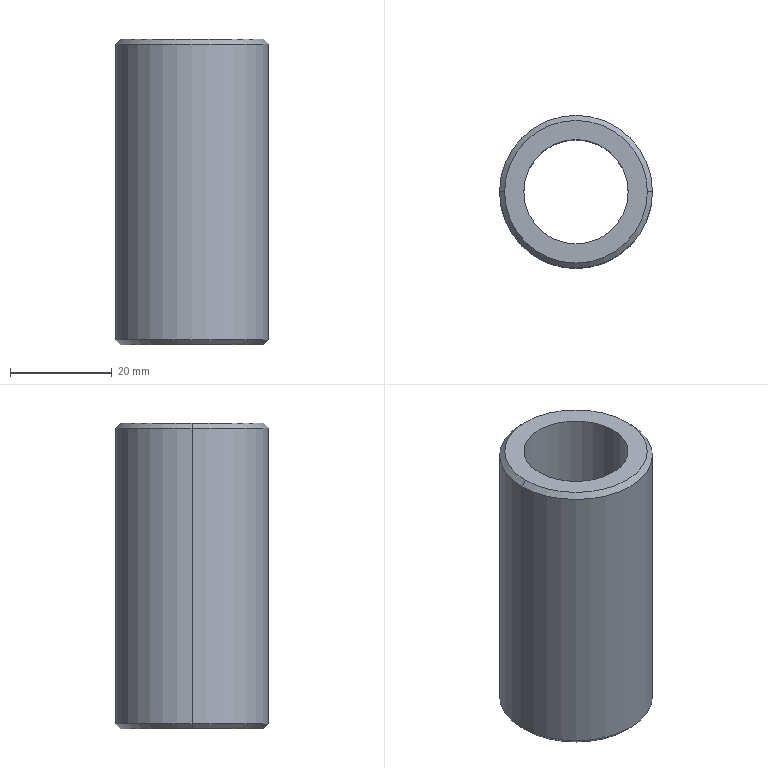Part | STEP file | Bushing_dia30_len60V11 | 1 solid | 10 faces | box 30 x 30 x 60 mm | volume 22516 mm3 | cone 4 | cylinder 4 | plane 2 | commonest cylinder face diameters 20.5 x2 30 x2
STEP:
#1=CARTESIAN_POINT('',(0.,0.,0.));
#2=DIRECTION('',(0.,0.,1.));
#3=DIRECTION('',(1.,0.,0.));
#4=AXIS2_PLACEMENT_3D('',#1,#2,#3);
#5=CARTESIAN_POINT('',(14.,0.,60.));
#6=VERTEX_POINT('',#5);
#7=CARTESIAN_POINT('',(-14.,0.,60.));
#8=VERTEX_POINT('',#7);
#9=CARTESIAN_POINT('',(0.,0.,60.));
#10=DIRECTION('',(0.,0.,1.));
#11=DIRECTION('',(1.,0.,0.));
#12=AXIS2_PLACEMENT_3D('',#9,#10,#11);
#13=CIRCLE('',#12,14.);
#14=CARTESIAN_POINT('',(0.,0.,60.));
#15=DIRECTION('',(0.,0.,-1.));
#16=DIRECTION('',(-1.,0.,0.));
#17=AXIS2_PLACEMENT_3D('',#14,#15,#16);
#18=CONICAL_SURFACE('',#17,14.,0.7854);
#19=CARTESIAN_POINT('',(3.142,0.));
#20=DIRECTION('',(-1.,0.));
#21=VECTOR('',#20,1.);
#22=LINE('',#19,#21);
#23=(GEOMETRIC_REPRESENTATION_CONTEXT(2)PARAMETRIC_REPRESENTATION_CONTEXT()REPRESENTATION_CONTEXT('',''));
#24=DEFINITIONAL_REPRESENTATION('',(#22),#23);
#25=PCURVE('',#18,#24);
#26=CARTESIAN_POINT('',(0.,0.,60.));
#27=DIRECTION('',(0.,0.,1.));
#28=DIRECTION('',(1.,0.,0.));
#29=AXIS2_PLACEMENT_3D('',#26,#27,#28);
#30=PLANE('',#29);
#31=CARTESIAN_POINT('',(0.,0.));
#32=DIRECTION('',(1.,0.));
#33=AXIS2_PLACEMENT_2D('',#31,#32);
#34=CIRCLE('',#33,14.);
#35=(GEOMETRIC_REPRESENTATION_CONTEXT(2)PARAMETRIC_REPRESENTATION_CONTEXT()REPRESENTATION_CONTEXT('',''));
#36=DEFINITIONAL_REPRESENTATION('',(#34),#35);
#37=PCURVE('',#30,#36);
#38=SURFACE_CURVE('',#13,(#25,#37),.PCURVE_S1.);
#39=EDGE_CURVE('',#6,#8,#38,.T.);
#40=ORIENTED_EDGE('',*,*,#39,.F.);
#41=CARTESIAN_POINT('',(15.,0.,59.));
#42=VERTEX_POINT('',#41);
#43=CARTESIAN_POINT('',(14.,0.,60.));
#44=DIRECTION('',(0.7071,0.,-0.7071));
#45=VECTOR('',#44,1.);
#46=LINE('',#43,#45);
#47=CARTESIAN_POINT('',(3.142,0.));
#48=DIRECTION('',(0.,1.));
#49=VECTOR('',#48,1.);
#50=LINE('',#47,#49);
#51=(GEOMETRIC_REPRESENTATION_CONTEXT(2)PARAMETRIC_REPRESENTATION_CONTEXT()REPRESENTATION_CONTEXT('',''));
#52=DEFINITIONAL_REPRESENTATION('',(#50),#51);
#53=PCURVE('',#18,#52);
#54=CARTESIAN_POINT('',(0.,0.,60.));
#55=DIRECTION('',(0.,0.,-1.));
#56=DIRECTION('',(-1.,0.,0.));
#57=AXIS2_PLACEMENT_3D('',#54,#55,#56);
#58=CONICAL_SURFACE('',#57,14.,0.7854);
#59=CARTESIAN_POINT('',(3.142,0.));
#60=DIRECTION('',(0.,1.));
#61=VECTOR('',#60,1.);
#62=LINE('',#59,#61);
#63=(GEOMETRIC_REPRESENTATION_CONTEXT(2)PARAMETRIC_REPRESENTATION_CONTEXT()REPRESENTATION_CONTEXT('',''));
#64=DEFINITIONAL_REPRESENTATION('',(#62),#63);
#65=PCURVE('',#58,#64);
#66=SURFACE_CURVE('',#46,(#53,#65),.PCURVE_S1.);
#67=EDGE_CURVE('',#6,#42,#66,.T.);
#68=ORIENTED_EDGE('',*,*,#67,.T.);
#69=CARTESIAN_POINT('',(-15.,0.,59.));
#70=VERTEX_POINT('',#69);
#71=CARTESIAN_POINT('',(0.,0.,59.));
#72=DIRECTION('',(0.,0.,-1.));
#73=DIRECTION('',(1.,0.,0.));
#74=AXIS2_PLACEMENT_3D('',#71,#72,#73);
#75=CIRCLE('',#74,15.);
#76=CARTESIAN_POINT('',(-3.142,1.));
#77=DIRECTION('',(1.,0.));
#78=VECTOR('',#77,1.);
#79=LINE('',#76,#78);
#80=(GEOMETRIC_REPRESENTATION_CONTEXT(2)PARAMETRIC_REPRESENTATION_CONTEXT()REPRESENTATION_CONTEXT('',''));
#81=DEFINITIONAL_REPRESENTATION('',(#79),#80);
#82=PCURVE('',#18,#81);
#83=CARTESIAN_POINT('',(0.,0.,60.));
#84=DIRECTION('',(0.,0.,-1.));
#85=DIRECTION('',(-1.,0.,0.));
#86=AXIS2_PLACEMENT_3D('',#83,#84,#85);
#87=CYLINDRICAL_SURFACE('',#86,15.);
#88=CARTESIAN_POINT('',(-3.142,1.));
#89=DIRECTION('',(1.,0.));
#90=VECTOR('',#89,1.);
#91=LINE('',#88,#90);
#92=(GEOMETRIC_REPRESENTATION_CONTEXT(2)PARAMETRIC_REPRESENTATION_CONTEXT()REPRESENTATION_CONTEXT('',''));
#93=DEFINITIONAL_REPRESENTATION('',(#91),#92);
#94=PCURVE('',#87,#93);
#95=SURFACE_CURVE('',#75,(#82,#94),.PCURVE_S1.);
#96=EDGE_CURVE('',#70,#42,#95,.T.);
#97=ORIENTED_EDGE('',*,*,#96,.F.);
#98=CARTESIAN_POINT('',(-14.,0.,60.));
#99=DIRECTION('',(-0.7071,0.,-0.7071));
#100=VECTOR('',#99,1.);
#101=LINE('',#98,#100);
#102=CARTESIAN_POINT('',(0.,0.));
#103=DIRECTION('',(0.,1.));
#104=VECTOR('',#103,1.);
#105=LINE('',#102,#104);
#106=(GEOMETRIC_REPRESENTATION_CONTEXT(2)PARAMETRIC_REPRESENTATION_CONTEXT()REPRESENTATION_CONTEXT('',''));
#107=DEFINITIONAL_REPRESENTATION('',(#105),#106);
#108=PCURVE('',#18,#107);
#109=CARTESIAN_POINT('',(6.283,0.));
#110=DIRECTION('',(0.,1.));
#111=VECTOR('',#110,1.);
#112=LINE('',#109,#111);
#113=(GEOMETRIC_REPRESENTATION_CONTEXT(2)PARAMETRIC_REPRESENTATION_CONTEXT()REPRESENTATION_CONTEXT('',''));
#114=DEFINITIONAL_REPRESENTATION('',(#112),#113);
#115=PCURVE('',#58,#114);
#116=SURFACE_CURVE('',#101,(#108,#115),.PCURVE_S1.);
#117=EDGE_CURVE('',#8,#70,#116,.T.);
#118=ORIENTED_EDGE('',*,*,#117,.F.);
#119=EDGE_LOOP('',(#40,#68,#97,#118));
#120=FACE_BOUND('',#119,.T.);
#121=ADVANCED_FACE('',(#120),#18,.T.);
#122=CARTESIAN_POINT('',(-14.,0.,0.));
#123=VERTEX_POINT('',#122);
#124=CARTESIAN_POINT('',(14.,0.,0.));
#125=VERTEX_POINT('',#124);
#126=CARTESIAN_POINT('',(0.,0.,0.));
#127=DIRECTION('',(0.,0.,-1.));
#128=DIRECTION('',(1.,0.,0.));
#129=AXIS2_PLACEMENT_3D('',#126,#127,#128);
#130=CIRCLE('',#129,14.);
#131=CARTESIAN_POINT('',(0.,0.,1.));
#132=DIRECTION('',(0.,0.,1.));
#133=DIRECTION('',(1.,0.,0.));
#134=AXIS2_PLACEMENT_3D('',#131,#132,#133);
#135=CONICAL_SURFACE('',#134,15.,0.7854);
#136=CARTESIAN_POINT('',(6.283,-1.));
#137=DIRECTION('',(-1.,0.));
#138=VECTOR('',#137,1.);
#139=LINE('',#136,#138);
#140=(GEOMETRIC_REPRESENTATION_CONTEXT(2)PARAMETRIC_REPRESENTATION_CONTEXT()REPRESENTATION_CONTEXT('',''));
#141=DEFINITIONAL_REPRESENTATION('',(#139),#140);
#142=PCURVE('',#135,#141);
#143=CARTESIAN_POINT('',(0.,0.,0.));
#144=DIRECTION('',(0.,0.,1.));
#145=DIRECTION('',(1.,0.,0.));
#146=AXIS2_PLACEMENT_3D('',#143,#144,#145);
#147=PLANE('',#146);
#148=CARTESIAN_POINT('',(14.,0.));
#149=CARTESIAN_POINT('',(14.,-24.249));
#150=CARTESIAN_POINT('',(-7.,-12.124));
#151=CARTESIAN_POINT('',(-28.,0.));
#152=CARTESIAN_POINT('',(-7.,12.124));
#153=CARTESIAN_POINT('',(14.,24.249));
#154=CARTESIAN_POINT('',(14.,0.));
#155=(BOUNDED_CURVE()B_SPLINE_CURVE(2,(#148,#149,#150,#151,#152,#153,#154),.UNSPECIFIED.,.T.,.F.)B_SPLINE_CURVE_WITH_KNOTS((1,2,2,2,2,1),(-2.094,0.,2.094,4.189,6.283,8.378),.UNSPECIFIED.)CURVE()GEOMETRIC_REPRESENTATION_ITEM()RATIONAL_B_SPLINE_CURVE((1.,0.5,1.,0.5,1.,0.5,1.))REPRESENTATION_ITEM(''));
#156=(GEOMETRIC_REPRESENTATION_CONTEXT(2)PARAMETRIC_REPRESENTATION_CONTEXT()REPRESENTATION_CONTEXT('',''));
#157=DEFINITIONAL_REPRESENTATION('',(#155),#156);
#158=PCURVE('',#147,#157);
#159=SURFACE_CURVE('',#130,(#142,#158),.PCURVE_S1.);
#160=EDGE_CURVE('',#123,#125,#159,.T.);
#161=ORIENTED_EDGE('',*,*,#160,.F.);
#162=CARTESIAN_POINT('',(-15.,0.,1.));
#163=VERTEX_POINT('',#162);
#164=CARTESIAN_POINT('',(-15.,0.,1.));
#165=DIRECTION('',(-0.7071,0.,0.7071));
#166=VECTOR('',#165,1.);
#167=LINE('',#164,#166);
#168=CARTESIAN_POINT('',(3.142,0.));
#169=DIRECTION('',(0.,1.));
#170=VECTOR('',#169,1.);
#171=LINE('',#168,#170);
#172=(GEOMETRIC_REPRESENTATION_CONTEXT(2)PARAMETRIC_REPRESENTATION_CONTEXT()REPRESENTATION_CONTEXT('',''));
#173=DEFINITIONAL_REPRESENTATION('',(#171),#172);
#174=PCURVE('',#135,#173);
#175=CARTESIAN_POINT('',(0.,0.,1.));
#176=DIRECTION('',(0.,0.,1.));
#177=DIRECTION('',(1.,0.,0.));
#178=AXIS2_PLACEMENT_3D('',#175,#176,#177);
#179=CONICAL_SURFACE('',#178,15.,0.7854);
#180=CARTESIAN_POINT('',(3.142,0.));
#181=DIRECTION('',(0.,1.));
#182=VECTOR('',#181,1.);
#183=LINE('',#180,#182);
#184=(GEOMETRIC_REPRESENTATION_CONTEXT(2)PARAMETRIC_REPRESENTATION_CONTEXT()REPRESENTATION_CONTEXT('',''));
#185=DEFINITIONAL_REPRESENTATION('',(#183),#184);
#186=PCURVE('',#179,#185);
#187=SURFACE_CURVE('',#167,(#174,#186),.PCURVE_S1.);
#188=EDGE_CURVE('',#123,#163,#187,.T.);
#189=ORIENTED_EDGE('',*,*,#188,.T.);
#190=CARTESIAN_POINT('',(15.,0.,1.));
#191=VERTEX_POINT('',#190);
#192=CARTESIAN_POINT('',(0.,0.,1.));
#193=DIRECTION('',(0.,0.,1.));
#194=DIRECTION('',(1.,0.,0.));
#195=AXIS2_PLACEMENT_3D('',#192,#193,#194);
#196=CIRCLE('',#195,15.);
#197=CARTESIAN_POINT('',(0.,0.));
#198=DIRECTION('',(1.,0.));
#199=VECTOR('',#198,1.);
#200=LINE('',#197,#199);
#201=(GEOMETRIC_REPRESENTATION_CONTEXT(2)PARAMETRIC_REPRESENTATION_CONTEXT()REPRESENTATION_CONTEXT('',''));
#202=DEFINITIONAL_REPRESENTATION('',(#200),#201);
#203=PCURVE('',#135,#202);
#204=CARTESIAN_POINT('',(3.142,59.));
#205=DIRECTION('',(-1.,0.));
#206=VECTOR('',#205,1.);
#207=LINE('',#204,#206);
#208=(GEOMETRIC_REPRESENTATION_CONTEXT(2)PARAMETRIC_REPRESENTATION_CONTEXT()REPRESENTATION_CONTEXT('',''));
#209=DEFINITIONAL_REPRESENTATION('',(#207),#208);
#210=PCURVE('',#87,#209);
#211=SURFACE_CURVE('',#196,(#203,#210),.PCURVE_S1.);
#212=EDGE_CURVE('',#191,#163,#211,.T.);
#213=ORIENTED_EDGE('',*,*,#212,.F.);
#214=CARTESIAN_POINT('',(15.,0.,1.));
#215=DIRECTION('',(0.7071,0.,0.7071));
#216=VECTOR('',#215,1.);
#217=LINE('',#214,#216);
#218=CARTESIAN_POINT('',(0.,0.));
#219=DIRECTION('',(0.,1.));
#220=VECTOR('',#219,1.);
#221=LINE('',#218,#220);
#222=(GEOMETRIC_REPRESENTATION_CONTEXT(2)PARAMETRIC_REPRESENTATION_CONTEXT()REPRESENTATION_CONTEXT('',''));
#223=DEFINITIONAL_REPRESENTATION('',(#221),#222);
#224=PCURVE('',#135,#223);
#225=CARTESIAN_POINT('',(6.283,0.));
#226=DIRECTION('',(0.,1.));
#227=VECTOR('',#226,1.);
#228=LINE('',#225,#227);
#229=(GEOMETRIC_REPRESENTATION_CONTEXT(2)PARAMETRIC_REPRESENTATION_CONTEXT()REPRESENTATION_CONTEXT('',''));
#230=DEFINITIONAL_REPRESENTATION('',(#228),#229);
#231=PCURVE('',#179,#230);
#232=SURFACE_CURVE('',#217,(#224,#231),.PCURVE_S1.);
#233=EDGE_CURVE('',#125,#191,#232,.T.);
#234=ORIENTED_EDGE('',*,*,#233,.F.);
#235=EDGE_LOOP('',(#161,#189,#213,#234));
#236=FACE_BOUND('',#235,.T.);
#237=ADVANCED_FACE('',(#236),#135,.T.);
#238=CARTESIAN_POINT('',(-10.25,0.,60.));
#239=VERTEX_POINT('',#238);
#240=CARTESIAN_POINT('',(-10.25,0.,0.));
#241=VERTEX_POINT('',#240);
#242=CARTESIAN_POINT('',(-10.25,0.,60.));
#243=DIRECTION('',(0.,0.,-1.));
#244=VECTOR('',#243,1.);
#245=LINE('',#242,#244);
#246=CARTESIAN_POINT('',(0.,0.,60.));
#247=DIRECTION('',(0.,0.,-1.));
#248=DIRECTION('',(-1.,0.,0.));
#249=AXIS2_PLACEMENT_3D('',#246,#247,#248);
#250=CYLINDRICAL_SURFACE('',#249,10.25);
#251=CARTESIAN_POINT('',(6.283,0.));
#252=DIRECTION('',(0.,1.));
#253=VECTOR('',#252,1.);
#254=LINE('',#251,#253);
#255=(GEOMETRIC_REPRESENTATION_CONTEXT(2)PARAMETRIC_REPRESENTATION_CONTEXT()REPRESENTATION_CONTEXT('',''));
#256=DEFINITIONAL_REPRESENTATION('',(#254),#255);
#257=PCURVE('',#250,#256);
#258=CARTESIAN_POINT('',(0.,0.,60.));
#259=DIRECTION('',(0.,0.,-1.));
#260=DIRECTION('',(-1.,0.,0.));
#261=AXIS2_PLACEMENT_3D('',#258,#259,#260);
#262=CYLINDRICAL_SURFACE('',#261,10.25);
#263=CARTESIAN_POINT('',(0.,0.));
#264=DIRECTION('',(0.,1.));
#265=VECTOR('',#264,1.);
#266=LINE('',#263,#265);
#267=(GEOMETRIC_REPRESENTATION_CONTEXT(2)PARAMETRIC_REPRESENTATION_CONTEXT()REPRESENTATION_CONTEXT('',''));
#268=DEFINITIONAL_REPRESENTATION('',(#266),#267);
#269=PCURVE('',#262,#268);
#270=SURFACE_CURVE('',#245,(#257,#269),.PCURVE_S1.);
#271=EDGE_CURVE('',#239,#241,#270,.T.);
#272=ORIENTED_EDGE('',*,*,#271,.T.);
#273=CARTESIAN_POINT('',(10.25,0.,0.));
#274=VERTEX_POINT('',#273);
#275=CARTESIAN_POINT('',(0.,0.,0.));
#276=DIRECTION('',(0.,0.,1.));
#277=DIRECTION('',(1.,0.,0.));
#278=AXIS2_PLACEMENT_3D('',#275,#276,#277);
#279=CIRCLE('',#278,10.25);
#280=CARTESIAN_POINT('',(9.425,60.));
#281=DIRECTION('',(-1.,0.));
#282=VECTOR('',#281,1.);
#283=LINE('',#280,#282);
#284=(GEOMETRIC_REPRESENTATION_CONTEXT(2)PARAMETRIC_REPRESENTATION_CONTEXT()REPRESENTATION_CONTEXT('',''));
#285=DEFINITIONAL_REPRESENTATION('',(#283),#284);
#286=PCURVE('',#250,#285);
#287=CARTESIAN_POINT('',(0.,0.));
#288=DIRECTION('',(1.,0.));
#289=AXIS2_PLACEMENT_2D('',#287,#288);
#290=CIRCLE('',#289,10.25);
#291=(GEOMETRIC_REPRESENTATION_CONTEXT(2)PARAMETRIC_REPRESENTATION_CONTEXT()REPRESENTATION_CONTEXT('',''));
#292=DEFINITIONAL_REPRESENTATION('',(#290),#291);
#293=PCURVE('',#147,#292);
#294=SURFACE_CURVE('',#279,(#286,#293),.PCURVE_S1.);
#295=EDGE_CURVE('',#241,#274,#294,.T.);
#296=ORIENTED_EDGE('',*,*,#295,.T.);
#297=CARTESIAN_POINT('',(10.25,0.,60.));
#298=VERTEX_POINT('',#297);
#299=CARTESIAN_POINT('',(10.25,0.,60.));
#300=DIRECTION('',(0.,0.,-1.));
#301=VECTOR('',#300,1.);
#302=LINE('',#299,#301);
#303=CARTESIAN_POINT('',(3.142,0.));
#304=DIRECTION('',(0.,1.));
#305=VECTOR('',#304,1.);
#306=LINE('',#303,#305);
#307=(GEOMETRIC_REPRESENTATION_CONTEXT(2)PARAMETRIC_REPRESENTATION_CONTEXT()REPRESENTATION_CONTEXT('',''));
#308=DEFINITIONAL_REPRESENTATION('',(#306),#307);
#309=PCURVE('',#250,#308);
#310=CARTESIAN_POINT('',(3.142,0.));
#311=DIRECTION('',(0.,1.));
#312=VECTOR('',#311,1.);
#313=LINE('',#310,#312);
#314=(GEOMETRIC_REPRESENTATION_CONTEXT(2)PARAMETRIC_REPRESENTATION_CONTEXT()REPRESENTATION_CONTEXT('',''));
#315=DEFINITIONAL_REPRESENTATION('',(#313),#314);
#316=PCURVE('',#262,#315);
#317=SURFACE_CURVE('',#302,(#309,#316),.PCURVE_S1.);
#318=EDGE_CURVE('',#298,#274,#317,.T.);
#319=ORIENTED_EDGE('',*,*,#318,.F.);
#320=CARTESIAN_POINT('',(0.,0.,60.));
#321=DIRECTION('',(0.,0.,1.));
#322=DIRECTION('',(1.,0.,0.));
#323=AXIS2_PLACEMENT_3D('',#320,#321,#322);
#324=CIRCLE('',#323,10.25);
#325=CARTESIAN_POINT('',(9.425,0.));
#326=DIRECTION('',(-1.,0.));
#327=VECTOR('',#326,1.);
#328=LINE('',#325,#327);
#329=(GEOMETRIC_REPRESENTATION_CONTEXT(2)PARAMETRIC_REPRESENTATION_CONTEXT()REPRESENTATION_CONTEXT('',''));
#330=DEFINITIONAL_REPRESENTATION('',(#328),#329);
#331=PCURVE('',#250,#330);
#332=CARTESIAN_POINT('',(0.,0.));
#333=DIRECTION('',(1.,0.));
#334=AXIS2_PLACEMENT_2D('',#332,#333);
#335=CIRCLE('',#334,10.25);
#336=(GEOMETRIC_REPRESENTATION_CONTEXT(2)PARAMETRIC_REPRESENTATION_CONTEXT()REPRESENTATION_CONTEXT('',''));
#337=DEFINITIONAL_REPRESENTATION('',(#335),#336);
#338=PCURVE('',#30,#337);
#339=SURFACE_CURVE('',#324,(#331,#338),.PCURVE_S1.);
#340=EDGE_CURVE('',#239,#298,#339,.T.);
#341=ORIENTED_EDGE('',*,*,#340,.F.);
#342=EDGE_LOOP('',(#272,#296,#319,#341));
#343=FACE_BOUND('',#342,.F.);
#344=ADVANCED_FACE('',(#343),#250,.F.);
#345=ORIENTED_EDGE('',*,*,#96,.T.);
#346=CARTESIAN_POINT('',(15.,0.,60.));
#347=DIRECTION('',(0.,0.,-1.));
#348=VECTOR('',#347,1.);
#349=LINE('',#346,#348);
#350=CARTESIAN_POINT('',(3.142,0.));
#351=DIRECTION('',(0.,1.));
#352=VECTOR('',#351,1.);
#353=LINE('',#350,#352);
#354=(GEOMETRIC_REPRESENTATION_CONTEXT(2)PARAMETRIC_REPRESENTATION_CONTEXT()REPRESENTATION_CONTEXT('',''));
#355=DEFINITIONAL_REPRESENTATION('',(#353),#354);
#356=PCURVE('',#87,#355);
#357=CARTESIAN_POINT('',(0.,0.,60.));
#358=DIRECTION('',(0.,0.,-1.));
#359=DIRECTION('',(-1.,0.,0.));
#360=AXIS2_PLACEMENT_3D('',#357,#358,#359);
#361=CYLINDRICAL_SURFACE('',#360,15.);
#362=CARTESIAN_POINT('',(3.142,0.));
#363=DIRECTION('',(0.,1.));
#364=VECTOR('',#363,1.);
#365=LINE('',#362,#364);
#366=(GEOMETRIC_REPRESENTATION_CONTEXT(2)PARAMETRIC_REPRESENTATION_CONTEXT()REPRESENTATION_CONTEXT('',''));
#367=DEFINITIONAL_REPRESENTATION('',(#365),#366);
#368=PCURVE('',#361,#367);
#369=SURFACE_CURVE('',#349,(#356,#368),.PCURVE_S1.);
#370=EDGE_CURVE('',#42,#191,#369,.T.);
#371=ORIENTED_EDGE('',*,*,#370,.T.);
#372=ORIENTED_EDGE('',*,*,#212,.T.);
#373=CARTESIAN_POINT('',(-15.,0.,60.));
#374=DIRECTION('',(0.,0.,-1.));
#375=VECTOR('',#374,1.);
#376=LINE('',#373,#375);
#377=CARTESIAN_POINT('',(0.,0.));
#378=DIRECTION('',(0.,1.));
#379=VECTOR('',#378,1.);
#380=LINE('',#377,#379);
#381=(GEOMETRIC_REPRESENTATION_CONTEXT(2)PARAMETRIC_REPRESENTATION_CONTEXT()REPRESENTATION_CONTEXT('',''));
#382=DEFINITIONAL_REPRESENTATION('',(#380),#381);
#383=PCURVE('',#87,#382);
#384=CARTESIAN_POINT('',(6.283,0.));
#385=DIRECTION('',(0.,1.));
#386=VECTOR('',#385,1.);
#387=LINE('',#384,#386);
#388=(GEOMETRIC_REPRESENTATION_CONTEXT(2)PARAMETRIC_REPRESENTATION_CONTEXT()REPRESENTATION_CONTEXT('',''));
#389=DEFINITIONAL_REPRESENTATION('',(#387),#388);
#390=PCURVE('',#361,#389);
#391=SURFACE_CURVE('',#376,(#383,#390),.PCURVE_S1.);
#392=EDGE_CURVE('',#70,#163,#391,.T.);
#393=ORIENTED_EDGE('',*,*,#392,.F.);
#394=EDGE_LOOP('',(#345,#371,#372,#393));
#395=FACE_BOUND('',#394,.T.);
#396=ADVANCED_FACE('',(#395),#87,.T.);
#397=CARTESIAN_POINT('',(0.,0.,60.));
#398=DIRECTION('',(0.,0.,1.));
#399=DIRECTION('',(1.,0.,0.));
#400=AXIS2_PLACEMENT_3D('',#397,#398,#399);
#401=CIRCLE('',#400,14.);
#402=CARTESIAN_POINT('',(0.,0.));
#403=DIRECTION('',(1.,0.));
#404=AXIS2_PLACEMENT_2D('',#402,#403);
#405=CIRCLE('',#404,14.);
#406=(GEOMETRIC_REPRESENTATION_CONTEXT(2)PARAMETRIC_REPRESENTATION_CONTEXT()REPRESENTATION_CONTEXT('',''));
#407=DEFINITIONAL_REPRESENTATION('',(#405),#406);
#408=PCURVE('',#30,#407);
#409=CARTESIAN_POINT('',(9.425,0.));
#410=DIRECTION('',(-1.,0.));
#411=VECTOR('',#410,1.);
#412=LINE('',#409,#411);
#413=(GEOMETRIC_REPRESENTATION_CONTEXT(2)PARAMETRIC_REPRESENTATION_CONTEXT()REPRESENTATION_CONTEXT('',''));
#414=DEFINITIONAL_REPRESENTATION('',(#412),#413);
#415=PCURVE('',#58,#414);
#416=SURFACE_CURVE('',#401,(#408,#415),.PCURVE_S1.);
#417=EDGE_CURVE('',#8,#6,#416,.T.);
#418=ORIENTED_EDGE('',*,*,#417,.T.);
#419=ORIENTED_EDGE('',*,*,#39,.T.);
#420=EDGE_LOOP('',(#418,#419));
#421=FACE_BOUND('',#420,.T.);
#422=ORIENTED_EDGE('',*,*,#340,.F.);
#423=CARTESIAN_POINT('',(0.,0.,60.));
#424=DIRECTION('',(0.,0.,1.));
#425=DIRECTION('',(1.,0.,0.));
#426=AXIS2_PLACEMENT_3D('',#423,#424,#425);
#427=CIRCLE('',#426,10.25);
#428=CARTESIAN_POINT('',(0.,0.));
#429=DIRECTION('',(1.,0.));
#430=AXIS2_PLACEMENT_2D('',#428,#429);
#431=CIRCLE('',#430,10.25);
#432=(GEOMETRIC_REPRESENTATION_CONTEXT(2)PARAMETRIC_REPRESENTATION_CONTEXT()REPRESENTATION_CONTEXT('',''));
#433=DEFINITIONAL_REPRESENTATION('',(#431),#432);
#434=PCURVE('',#30,#433);
#435=CARTESIAN_POINT('',(3.142,0.));
#436=DIRECTION('',(-1.,0.));
#437=VECTOR('',#436,1.);
#438=LINE('',#435,#437);
#439=(GEOMETRIC_REPRESENTATION_CONTEXT(2)PARAMETRIC_REPRESENTATION_CONTEXT()REPRESENTATION_CONTEXT('',''));
#440=DEFINITIONAL_REPRESENTATION('',(#438),#439);
#441=PCURVE('',#262,#440);
#442=SURFACE_CURVE('',#427,(#434,#441),.PCURVE_S1.);
#443=EDGE_CURVE('',#298,#239,#442,.T.);
#444=ORIENTED_EDGE('',*,*,#443,.F.);
#445=EDGE_LOOP('',(#422,#444));
#446=FACE_BOUND('',#445,.T.);
#447=ADVANCED_FACE('',(#421,#446),#30,.T.);
#448=CARTESIAN_POINT('',(0.,0.,0.));
#449=DIRECTION('',(0.,0.,-1.));
#450=DIRECTION('',(1.,0.,0.));
#451=AXIS2_PLACEMENT_3D('',#448,#449,#450);
#452=CIRCLE('',#451,14.);
#453=CARTESIAN_POINT('',(14.,0.));
#454=CARTESIAN_POINT('',(14.,-24.249));
#455=CARTESIAN_POINT('',(-7.,-12.124));
#456=CARTESIAN_POINT('',(-28.,0.));
#457=CARTESIAN_POINT('',(-7.,12.124));
#458=CARTESIAN_POINT('',(14.,24.249));
#459=CARTESIAN_POINT('',(14.,0.));
#460=(BOUNDED_CURVE()B_SPLINE_CURVE(2,(#453,#454,#455,#456,#457,#458,#459),.UNSPECIFIED.,.T.,.F.)B_SPLINE_CURVE_WITH_KNOTS((1,2,2,2,2,1),(-2.094,0.,2.094,4.189,6.283,8.378),.UNSPECIFIED.)CURVE()GEOMETRIC_REPRESENTATION_ITEM()RATIONAL_B_SPLINE_CURVE((1.,0.5,1.,0.5,1.,0.5,1.))REPRESENTATION_ITEM(''));
#461=(GEOMETRIC_REPRESENTATION_CONTEXT(2)PARAMETRIC_REPRESENTATION_CONTEXT()REPRESENTATION_CONTEXT('',''));
#462=DEFINITIONAL_REPRESENTATION('',(#460),#461);
#463=PCURVE('',#147,#462);
#464=CARTESIAN_POINT('',(6.283,-1.));
#465=DIRECTION('',(-1.,0.));
#466=VECTOR('',#465,1.);
#467=LINE('',#464,#466);
#468=(GEOMETRIC_REPRESENTATION_CONTEXT(2)PARAMETRIC_REPRESENTATION_CONTEXT()REPRESENTATION_CONTEXT('',''));
#469=DEFINITIONAL_REPRESENTATION('',(#467),#468);
#470=PCURVE('',#179,#469);
#471=SURFACE_CURVE('',#452,(#463,#470),.PCURVE_S1.);
#472=EDGE_CURVE('',#125,#123,#471,.T.);
#473=ORIENTED_EDGE('',*,*,#472,.T.);
#474=ORIENTED_EDGE('',*,*,#160,.T.);
#475=EDGE_LOOP('',(#473,#474));
#476=FACE_BOUND('',#475,.T.);
#477=ORIENTED_EDGE('',*,*,#295,.T.);
#478=CARTESIAN_POINT('',(0.,0.,0.));
#479=DIRECTION('',(0.,0.,1.));
#480=DIRECTION('',(1.,0.,0.));
#481=AXIS2_PLACEMENT_3D('',#478,#479,#480);
#482=CIRCLE('',#481,10.25);
#483=CARTESIAN_POINT('',(0.,0.));
#484=DIRECTION('',(1.,0.));
#485=AXIS2_PLACEMENT_2D('',#483,#484);
#486=CIRCLE('',#485,10.25);
#487=(GEOMETRIC_REPRESENTATION_CONTEXT(2)PARAMETRIC_REPRESENTATION_CONTEXT()REPRESENTATION_CONTEXT('',''));
#488=DEFINITIONAL_REPRESENTATION('',(#486),#487);
#489=PCURVE('',#147,#488);
#490=CARTESIAN_POINT('',(3.142,60.));
#491=DIRECTION('',(-1.,0.));
#492=VECTOR('',#491,1.);
#493=LINE('',#490,#492);
#494=(GEOMETRIC_REPRESENTATION_CONTEXT(2)PARAMETRIC_REPRESENTATION_CONTEXT()REPRESENTATION_CONTEXT('',''));
#495=DEFINITIONAL_REPRESENTATION('',(#493),#494);
#496=PCURVE('',#262,#495);
#497=SURFACE_CURVE('',#482,(#489,#496),.PCURVE_S1.);
#498=EDGE_CURVE('',#274,#241,#497,.T.);
#499=ORIENTED_EDGE('',*,*,#498,.T.);
#500=EDGE_LOOP('',(#477,#499));
#501=FACE_BOUND('',#500,.T.);
#502=ADVANCED_FACE('',(#476,#501),#147,.F.);
#503=ORIENTED_EDGE('',*,*,#370,.F.);
#504=CARTESIAN_POINT('',(0.,0.,59.));
#505=DIRECTION('',(0.,0.,-1.));
#506=DIRECTION('',(1.,0.,0.));
#507=AXIS2_PLACEMENT_3D('',#504,#505,#506);
#508=CIRCLE('',#507,15.);
#509=CARTESIAN_POINT('',(3.142,1.));
#510=DIRECTION('',(1.,0.));
#511=VECTOR('',#510,1.);
#512=LINE('',#509,#511);
#513=(GEOMETRIC_REPRESENTATION_CONTEXT(2)PARAMETRIC_REPRESENTATION_CONTEXT()REPRESENTATION_CONTEXT('',''));
#514=DEFINITIONAL_REPRESENTATION('',(#512),#513);
#515=PCURVE('',#361,#514);
#516=CARTESIAN_POINT('',(3.142,1.));
#517=DIRECTION('',(1.,0.));
#518=VECTOR('',#517,1.);
#519=LINE('',#516,#518);
#520=(GEOMETRIC_REPRESENTATION_CONTEXT(2)PARAMETRIC_REPRESENTATION_CONTEXT()REPRESENTATION_CONTEXT('',''));
#521=DEFINITIONAL_REPRESENTATION('',(#519),#520);
#522=PCURVE('',#58,#521);
#523=SURFACE_CURVE('',#508,(#515,#522),.PCURVE_S1.);
#524=EDGE_CURVE('',#42,#70,#523,.T.);
#525=ORIENTED_EDGE('',*,*,#524,.T.);
#526=ORIENTED_EDGE('',*,*,#392,.T.);
#527=CARTESIAN_POINT('',(0.,0.,1.));
#528=DIRECTION('',(0.,0.,1.));
#529=DIRECTION('',(1.,0.,0.));
#530=AXIS2_PLACEMENT_3D('',#527,#528,#529);
#531=CIRCLE('',#530,15.);
#532=CARTESIAN_POINT('',(9.425,59.));
#533=DIRECTION('',(-1.,0.));
#534=VECTOR('',#533,1.);
#535=LINE('',#532,#534);
#536=(GEOMETRIC_REPRESENTATION_CONTEXT(2)PARAMETRIC_REPRESENTATION_CONTEXT()REPRESENTATION_CONTEXT('',''));
#537=DEFINITIONAL_REPRESENTATION('',(#535),#536);
#538=PCURVE('',#361,#537);
#539=CARTESIAN_POINT('',(0.,0.));
#540=DIRECTION('',(1.,0.));
#541=VECTOR('',#540,1.);
#542=LINE('',#539,#541);
#543=(GEOMETRIC_REPRESENTATION_CONTEXT(2)PARAMETRIC_REPRESENTATION_CONTEXT()REPRESENTATION_CONTEXT('',''));
#544=DEFINITIONAL_REPRESENTATION('',(#542),#543);
#545=PCURVE('',#179,#544);
#546=SURFACE_CURVE('',#531,(#538,#545),.PCURVE_S1.);
#547=EDGE_CURVE('',#163,#191,#546,.T.);
#548=ORIENTED_EDGE('',*,*,#547,.T.);
#549=EDGE_LOOP('',(#503,#525,#526,#548));
#550=FACE_BOUND('',#549,.T.);
#551=ADVANCED_FACE('',(#550),#361,.T.);
#552=ORIENTED_EDGE('',*,*,#498,.T.);
#553=ORIENTED_EDGE('',*,*,#271,.F.);
#554=ORIENTED_EDGE('',*,*,#443,.F.);
#555=ORIENTED_EDGE('',*,*,#318,.T.);
#556=EDGE_LOOP('',(#552,#553,#554,#555));
#557=FACE_BOUND('',#556,.F.);
#558=ADVANCED_FACE('',(#557),#262,.F.);
#559=ORIENTED_EDGE('',*,*,#188,.F.);
#560=ORIENTED_EDGE('',*,*,#472,.F.);
#561=ORIENTED_EDGE('',*,*,#233,.T.);
#562=ORIENTED_EDGE('',*,*,#547,.F.);
#563=EDGE_LOOP('',(#559,#560,#561,#562));
#564=FACE_BOUND('',#563,.T.);
#565=ADVANCED_FACE('',(#564),#179,.T.);
#566=ORIENTED_EDGE('',*,*,#67,.F.);
#567=ORIENTED_EDGE('',*,*,#417,.F.);
#568=ORIENTED_EDGE('',*,*,#117,.T.);
#569=ORIENTED_EDGE('',*,*,#524,.F.);
#570=EDGE_LOOP('',(#566,#567,#568,#569));
#571=FACE_BOUND('',#570,.T.);
#572=ADVANCED_FACE('',(#571),#58,.T.);
#573=CLOSED_SHELL('',(#121,#237,#344,#396,#447,#502,#551,#558,#565,#572));
#574=MANIFOLD_SOLID_BREP('',#573);
#575=(LENGTH_UNIT()NAMED_UNIT(*)SI_UNIT(.MILLI.,.METRE.));
#576=UNCERTAINTY_MEASURE_WITH_UNIT(LENGTH_MEASURE(0.0000001),#575,'','');
#577=(NAMED_UNIT(*)PLANE_ANGLE_UNIT()SI_UNIT($,.RADIAN.));
#578=(NAMED_UNIT(*)SI_UNIT($,.STERADIAN.)SOLID_ANGLE_UNIT());
#579=(GEOMETRIC_REPRESENTATION_CONTEXT(3)GLOBAL_UNCERTAINTY_ASSIGNED_CONTEXT((#576))GLOBAL_UNIT_ASSIGNED_CONTEXT((#575,#577,#578))REPRESENTATION_CONTEXT('',''));
#580=ADVANCED_BREP_SHAPE_REPRESENTATION('',(#4,#574),#579);